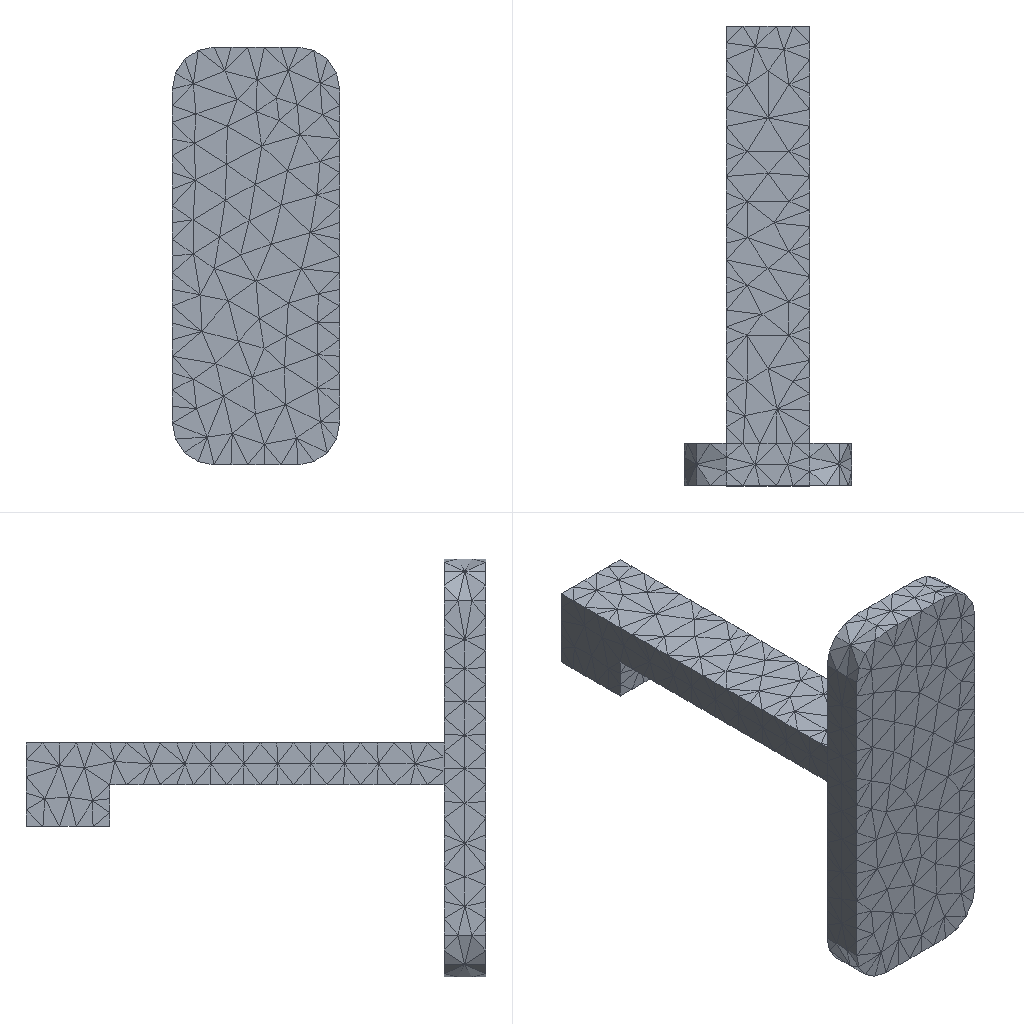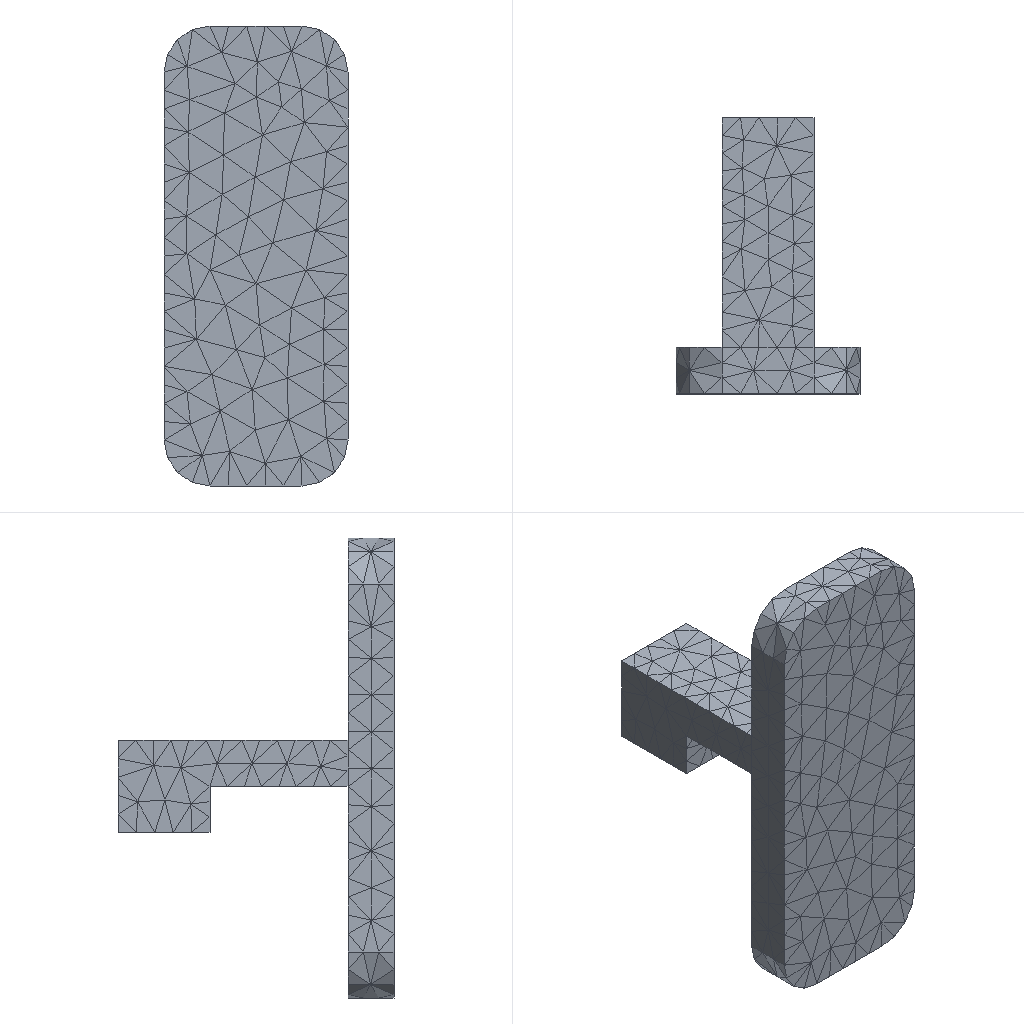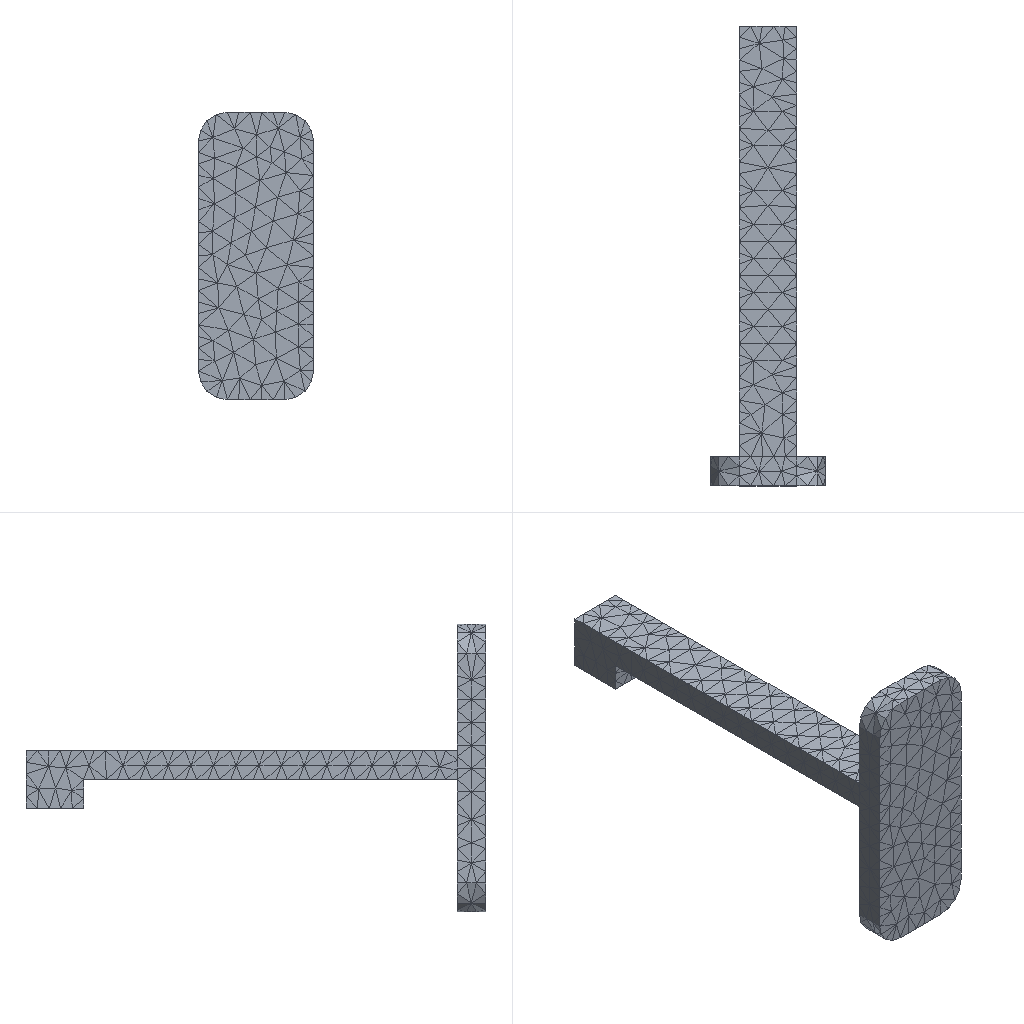Simulation study | ansys workbench
Set-up summary:
category,name,step,type,value,unit,region
solver,ansys_workbench
units,mm-N-s-tonne (MPa),,stated,"/units,MPA"
analysis,deck-1/LS1,,static
load_step,deck-1/LS1,deck-1/LS1,static,nsubst=1; time=1
analysis,deck-2/LS1,,static
load_step,deck-2/LS1,deck-2/LS1,static,nsubst=1; time=1
analysis,deck-3/LS1,,static
load_step,deck-3/LS1,deck-3/LS1,static,nsubst=1; time=1
analysis,deck-4/LS1,,static
load_step,deck-4/LS1,deck-4/LS1,static,nsubst=1; time=1
analysis,deck-5/LS1,,static
load_step,deck-5/LS1,deck-5/LS1,static,nsubst=1; time=1
mesh,deck-1.dat,,nodes,3511
mesh,deck-1.dat,,elements,1778
element_type,SOLID187,,,1750,,deck-1.dat
element_type,SURF154,,,28,,deck-1.dat
mesh,deck-2.dat,,nodes,2968
mesh,deck-2.dat,,elements,1500
element_type,SOLID187,,,1472,,deck-2.dat
element_type,SURF154,,,28,,deck-2.dat
mesh,deck-3.dat,,nodes,4033
mesh,deck-3.dat,,elements,2010
element_type,SOLID187,,,1982,,deck-3.dat
element_type,SURF154,,,28,,deck-3.dat
mesh,deck-4.dat,,nodes,4502
mesh,deck-4.dat,,elements,2218
element_type,SOLID187,,,2190,,deck-4.dat
element_type,SURF154,,,28,,deck-4.dat
mesh,deck-5.dat,,nodes,2664
mesh,deck-5.dat,,elements,1350
element_type,SOLID187,,,1322,,deck-5.dat
element_type,SURF154,,,28,,deck-5.dat
material,Structural Steel,,E,200000,tonne s^-2 mm^-1
material,Structural Steel,,nu,0.3
material,Structural Steel,,density,7.85e-09,tonne mm^-3
material,Structural Steel,,conductivity,60.5,tonne mm s^-3 C^-1
material,Structural Steel,,specific_heat,4.34e+08,mm^2 s^-2 C^-1
material,Structural Steel,,cte,1.2e-05,C^-1
material,Structural Steel,,permeability,10000
material,Structural Steel,,resistivity,0.00017,ohm mm
material,304,,E,200000,tonne s^-2 mm^-1
material,304,,nu,0.3
material,304,,density,7.85e-09,tonne mm^-3
material,304,,conductivity,60.5,tonne mm s^-3 C^-1
material,304,,specific_heat,4.34e+08,mm^2 s^-2 C^-1
material,304,,cte,1.2e-05,C^-1
material,304,,permeability,10000
material,304,,resistivity,0.00017,ohm mm
material,304,,E,200000,tonne s^-2 mm^-1
material,304,,nu,0.3
material,304,,density,7.85e-09,tonne mm^-3
material,304,,conductivity,60.5,tonne mm s^-3 C^-1
material,304,,specific_heat,4.34e+08,mm^2 s^-2 C^-1
material,304,,cte,1.2e-05,C^-1
material,304,,permeability,10000
material,304,,resistivity,0.00017,ohm mm
load,Define Force Using Surface Effect Elements,deck-1/LS1,surface-effect pres face 3,5,,SURF154 #2
load,Define Force Using Surface Effect Elements,deck-2/LS1,surface-effect pres face 3,5,,SURF154 #2
load,Define Force Using Surface Effect Elements,deck-3/LS1,surface-effect pres face 3,5,,SURF154 #2
load,Define Force Using Surface Effect Elements,deck-4/LS1,surface-effect pres face 3,5,,SURF154 #2
load,Define Force Using Surface Effect Elements,deck-5/LS1,surface-effect pres face 3,5,,SURF154 #2
bc,Fixed Supports,deck-1/model,fixed,[dofs=ALL],,_FIXEDSU
bc,Fixed Supports,deck-2/model,fixed,[dofs=ALL],,_FIXEDSU
bc,Fixed Supports,deck-3/model,fixed,[dofs=ALL],,_FIXEDSU
bc,Fixed Supports,deck-4/model,fixed,[dofs=ALL],,_FIXEDSU
bc,Fixed Supports,deck-5/model,fixed,[dofs=ALL],,_FIXEDSU
named_set,_FIXEDSU,,node,431
named_set,_FIXEDSU,,node,431
named_set,_FIXEDSU,,node,431
named_set,_FIXEDSU,,node,431
named_set,_FIXEDSU,,node,431
Results summary:
result,analyses[0].index,,,1
result,analyses[0].system,,,SYS
result,analyses[0].deck,,,deck-1.dat
result,analyses[0].solve_status,,,completed
result,analyses[0].analysis_type,,,static
result,analyses[0].physics,,,mechanical
result,analyses[0].unit_system,,,"NMM: mm, ton, N, s, mV, mA, degC"
result,analyses[0].n_sets,,,1
result,analyses[0].load_steps[0].set,set=1,,1
result,analyses[0].load_steps[0].time_or_freq,set=1,,1
result,analyses[0].load_steps[0].max_displacement_magnitude,set=1,,0.9288
result,analyses[0].load_steps[0].max_von_mises_nodal,set=1,,553.976
result,analyses[0].load_steps[0].reaction_force_sum_xyz[1],set=1,,3.53586e-09
result,analyses[0].load_steps[0].reaction_force_sum_xyz[2],set=1,,1.04197e-10
result,analyses[0].load_steps[0].reaction_force_sum_xyz[3],set=1,,-500
result,analyses[1].index,,,2
result,analyses[1].system,,,SYS-1
result,analyses[1].deck,,,deck-2.dat
result,analyses[1].solve_status,,,completed
result,analyses[1].analysis_type,,,static
result,analyses[1].physics,,,mechanical
result,analyses[1].unit_system,,,"NMM: mm, ton, N, s, mV, mA, degC"
result,analyses[1].n_sets,,,1
result,analyses[1].load_steps[0].set,set=1,,1
result,analyses[1].load_steps[0].time_or_freq,set=1,,1
result,analyses[1].load_steps[0].max_displacement_magnitude,set=1,,0.1102
result,analyses[1].load_steps[0].max_von_mises_nodal,set=1,,235.984
result,analyses[1].load_steps[0].reaction_force_sum_xyz[1],set=1,,7.25724e-06
result,analyses[1].load_steps[0].reaction_force_sum_xyz[2],set=1,,3.42474e-06
result,analyses[1].load_steps[0].reaction_force_sum_xyz[3],set=1,,-500
result,analyses[2].index,,,3
result,analyses[2].system,,,SYS-2
result,analyses[2].deck,,,deck-3.dat
result,analyses[2].solve_status,,,completed
result,analyses[2].analysis_type,,,static
result,analyses[2].physics,,,mechanical
result,analyses[2].unit_system,,,"NMM: mm, ton, N, s, mV, mA, degC"
result,analyses[2].n_sets,,,1
result,analyses[2].load_steps[0].set,set=1,,1
result,analyses[2].load_steps[0].time_or_freq,set=1,,1
result,analyses[2].load_steps[0].max_displacement_magnitude,set=1,,3.205
result,analyses[2].load_steps[0].max_von_mises_nodal,set=1,,903.105
result,analyses[2].load_steps[0].reaction_force_sum_xyz[1],set=1,,1.41924e-07
result,analyses[2].load_steps[0].reaction_force_sum_xyz[2],set=1,,-1.13236e-07
result,analyses[2].load_steps[0].reaction_force_sum_xyz[3],set=1,,-500
result,analyses[3].index,,,4
result,analyses[3].system,,,SYS-3
result,analyses[3].deck,,,deck-4.dat
result,analyses[3].solve_status,,,completed
result,analyses[3].analysis_type,,,static
result,analyses[3].physics,,,mechanical
result,analyses[3].unit_system,,,"NMM: mm, ton, N, s, mV, mA, degC"
result,analyses[3].n_sets,,,1
result,analyses[3].load_steps[0].set,set=1,,1
result,analyses[3].load_steps[0].time_or_freq,set=1,,1
result,analyses[3].load_steps[0].max_displacement_magnitude,set=1,,7.685
result,analyses[3].load_steps[0].max_von_mises_nodal,set=1,,1202.09
result,analyses[3].load_steps[0].reaction_force_sum_xyz[1],set=1,,7.92352e-07
result,analyses[3].load_steps[0].reaction_force_sum_xyz[2],set=1,,-1.49288e-06
result,analyses[3].load_steps[0].reaction_force_sum_xyz[3],set=1,,-500
result,analyses[4].index,,,5
result,analyses[4].system,,,SYS-4
result,analyses[4].deck,,,deck-5.dat
result,analyses[4].solve_status,,,completed
result,analyses[4].analysis_type,,,static
result,analyses[4].physics,,,mechanical
result,analyses[4].unit_system,,,"NMM: mm, ton, N, s, mV, mA, degC"
result,analyses[4].n_sets,,,1
result,analyses[4].load_steps[0].set,set=1,,1
result,analyses[4].load_steps[0].time_or_freq,set=1,,1
result,analyses[4].load_steps[0].max_displacement_magnitude,set=1,,0.02655
result,analyses[4].load_steps[0].max_von_mises_nodal,set=1,,113.234
result,analyses[4].load_steps[0].reaction_force_sum_xyz[1],set=1,,8.7052e-10
result,analyses[4].load_steps[0].reaction_force_sum_xyz[2],set=1,,-8.82605e-12
result,analyses[4].load_steps[0].reaction_force_sum_xyz[3],set=1,,-500
result,geometry_export[0][0],,,1.step
result,geometry_export[0][1],,,ok
result,geometry_export[0][2],,,1
result,geometry_export[1][0],,,2.step
result,geometry_export[1][1],,,ok
result,geometry_export[1][2],,,1
result,geometry_export[2][0],,,3.step
result,geometry_export[2][1],,,ok
result,geometry_export[2][2],,,1
result,geometry_export[3][0],,,4.step
result,geometry_export[3][1],,,ok
result,geometry_export[3][2],,,1
result,geometry_export[4][0],,,5.step
result,geometry_export[4][1],,,ok
result,geometry_export[4][2],,,1